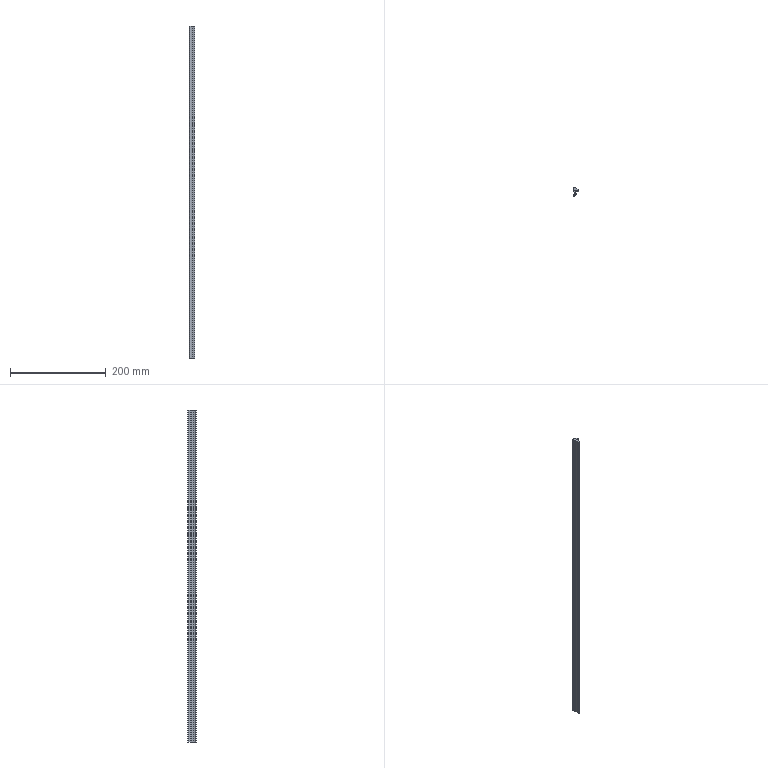Part | SolidWorks | features BaseBody 1, MoveFace 1 | 1 solid | 20 faces | box 10.8 x 17.5 x 692 mm | volume 54530 mm3 | cylinder 11 | plane 9 | commonest cylinder face diameters 1.6 x2 14 x2 0.4 x1 0.6 x1 0.8 x1 2.6 x1
STEP:
#1=CARTESIAN_POINT('',(-3.236,-11.055,592.));
#2=VERTEX_POINT('',#1);
#3=CARTESIAN_POINT('',(-4.3,-10.3,592.));
#4=VERTEX_POINT('',#3);
#5=CARTESIAN_POINT('',(-3.5,-10.3,592.));
#6=DIRECTION('',(0.,0.,-1.));
#7=DIRECTION('',(1.,0.,0.));
#8=AXIS2_PLACEMENT_3D('',#5,#6,#7);
#9=CIRCLE('',#8,0.8);
#10=EDGE_CURVE('',#2,#4,#9,.T.);
#11=ORIENTED_EDGE('',*,*,#10,.T.);
#12=CARTESIAN_POINT('',(-4.3,-10.3,-100.));
#13=VERTEX_POINT('',#12);
#14=CARTESIAN_POINT('',(-4.3,-10.3,-100.));
#15=DIRECTION('',(0.,0.,-1.));
#16=VECTOR('',#15,1000.);
#17=LINE('',#14,#16);
#18=EDGE_CURVE('',#4,#13,#17,.T.);
#19=ORIENTED_EDGE('',*,*,#18,.T.);
#20=CARTESIAN_POINT('',(-3.236,-11.055,-100.));
#21=VERTEX_POINT('',#20);
#22=CARTESIAN_POINT('',(-3.5,-10.3,-100.));
#23=DIRECTION('',(0.,0.,1.));
#24=DIRECTION('',(-1.,0.,0.));
#25=AXIS2_PLACEMENT_3D('',#22,#23,#24);
#26=CIRCLE('',#25,0.8);
#27=EDGE_CURVE('',#13,#21,#26,.T.);
#28=ORIENTED_EDGE('',*,*,#27,.T.);
#29=CARTESIAN_POINT('',(-3.236,-11.055,-100.));
#30=DIRECTION('',(0.,0.,-1.));
#31=VECTOR('',#30,1000.);
#32=LINE('',#29,#31);
#33=EDGE_CURVE('',#2,#21,#32,.T.);
#34=ORIENTED_EDGE('',*,*,#33,.F.);
#35=EDGE_LOOP('',(#11,#19,#28,#34));
#36=FACE_OUTER_BOUND('',#35,.T.);
#37=CARTESIAN_POINT('',(-3.5,-10.3,-100.));
#38=DIRECTION('',(0.,0.,-1.));
#39=DIRECTION('',(-1.,0.,0.));
#40=AXIS2_PLACEMENT_3D('',#37,#38,#39);
#41=CYLINDRICAL_SURFACE('',#40,0.8);
#42=ADVANCED_FACE('',(#36),#41,.T.);
#43=CARTESIAN_POINT('',(1.184,-6.397,-100.));
#44=VERTEX_POINT('',#43);
#45=CARTESIAN_POINT('',(-5.702,-4.29,-100.));
#46=DIRECTION('',(0.,0.,1.));
#47=DIRECTION('',(-1.,0.,0.));
#48=AXIS2_PLACEMENT_3D('',#45,#46,#47);
#49=CIRCLE('',#48,7.201);
#50=EDGE_CURVE('',#21,#44,#49,.T.);
#51=ORIENTED_EDGE('',*,*,#50,.T.);
#52=CARTESIAN_POINT('',(1.184,-6.397,592.));
#53=VERTEX_POINT('',#52);
#54=CARTESIAN_POINT('',(1.184,-6.397,-100.));
#55=DIRECTION('',(0.,0.,1.));
#56=VECTOR('',#55,1000.);
#57=LINE('',#54,#56);
#58=EDGE_CURVE('',#44,#53,#57,.T.);
#59=ORIENTED_EDGE('',*,*,#58,.T.);
#60=CARTESIAN_POINT('',(-5.702,-4.29,592.));
#61=DIRECTION('',(0.,0.,-1.));
#62=DIRECTION('',(1.,0.,0.));
#63=AXIS2_PLACEMENT_3D('',#60,#61,#62);
#64=CIRCLE('',#63,7.201);
#65=EDGE_CURVE('',#53,#2,#64,.T.);
#66=ORIENTED_EDGE('',*,*,#65,.T.);
#67=ORIENTED_EDGE('',*,*,#33,.T.);
#68=EDGE_LOOP('',(#51,#59,#66,#67));
#69=FACE_OUTER_BOUND('',#68,.T.);
#70=CARTESIAN_POINT('',(-5.702,-4.29,-100.));
#71=DIRECTION('',(0.,0.,-1.));
#72=DIRECTION('',(-1.,0.,0.));
#73=AXIS2_PLACEMENT_3D('',#70,#71,#72);
#74=CYLINDRICAL_SURFACE('',#73,7.201);
#75=ADVANCED_FACE('',(#69),#74,.T.);
#76=CARTESIAN_POINT('',(0.9,-6.,-100.));
#77=VERTEX_POINT('',#76);
#78=CARTESIAN_POINT('',(0.9,-6.3,-100.));
#79=DIRECTION('',(0.,0.,1.));
#80=DIRECTION('',(-1.,0.,0.));
#81=AXIS2_PLACEMENT_3D('',#78,#79,#80);
#82=CIRCLE('',#81,0.3);
#83=EDGE_CURVE('',#44,#77,#82,.T.);
#84=ORIENTED_EDGE('',*,*,#83,.T.);
#85=CARTESIAN_POINT('',(0.9,-6.,592.));
#86=VERTEX_POINT('',#85);
#87=CARTESIAN_POINT('',(0.9,-6.,-100.));
#88=DIRECTION('',(0.,0.,1.));
#89=VECTOR('',#88,1000.);
#90=LINE('',#87,#89);
#91=EDGE_CURVE('',#77,#86,#90,.T.);
#92=ORIENTED_EDGE('',*,*,#91,.T.);
#93=CARTESIAN_POINT('',(0.9,-6.3,592.));
#94=DIRECTION('',(0.,0.,-1.));
#95=DIRECTION('',(1.,0.,0.));
#96=AXIS2_PLACEMENT_3D('',#93,#94,#95);
#97=CIRCLE('',#96,0.3);
#98=EDGE_CURVE('',#86,#53,#97,.T.);
#99=ORIENTED_EDGE('',*,*,#98,.T.);
#100=ORIENTED_EDGE('',*,*,#58,.F.);
#101=EDGE_LOOP('',(#84,#92,#99,#100));
#102=FACE_OUTER_BOUND('',#101,.T.);
#103=CARTESIAN_POINT('',(0.9,-6.3,-100.));
#104=DIRECTION('',(0.,0.,-1.));
#105=DIRECTION('',(-1.,0.,0.));
#106=AXIS2_PLACEMENT_3D('',#103,#104,#105);
#107=CYLINDRICAL_SURFACE('',#106,0.3);
#108=ADVANCED_FACE('',(#102),#107,.T.);
#109=CARTESIAN_POINT('',(-2.5,-0.5,-100.));
#110=VERTEX_POINT('',#109);
#111=CARTESIAN_POINT('',(-2.5,-6.153,-100.));
#112=VERTEX_POINT('',#111);
#113=CARTESIAN_POINT('',(-2.5,-6.397,-100.));
#114=DIRECTION('',(0.,-1.,0.));
#115=VECTOR('',#114,1000.);
#116=LINE('',#113,#115);
#117=EDGE_CURVE('',#110,#112,#116,.T.);
#118=ORIENTED_EDGE('',*,*,#117,.F.);
#119=CARTESIAN_POINT('',(-4.2,1.695,-100.));
#120=VERTEX_POINT('',#119);
#121=CARTESIAN_POINT('',(-1.701,1.875,-100.));
#122=DIRECTION('',(0.,0.,1.));
#123=DIRECTION('',(-1.,0.,0.));
#124=AXIS2_PLACEMENT_3D('',#121,#122,#123);
#125=CIRCLE('',#124,2.506);
#126=EDGE_CURVE('',#120,#110,#125,.T.);
#127=ORIENTED_EDGE('',*,*,#126,.F.);
#128=CARTESIAN_POINT('',(-4.2,5.1,-100.));
#129=VERTEX_POINT('',#128);
#130=CARTESIAN_POINT('',(-4.2,-6.397,-100.));
#131=DIRECTION('',(0.,-1.,0.));
#132=VECTOR('',#131,1000.);
#133=LINE('',#130,#132);
#134=EDGE_CURVE('',#129,#120,#133,.T.);
#135=ORIENTED_EDGE('',*,*,#134,.F.);
#136=CARTESIAN_POINT('',(-2.892,6.4,-100.));
#137=VERTEX_POINT('',#136);
#138=CARTESIAN_POINT('',(-2.9,5.1,-100.));
#139=DIRECTION('',(0.,0.,1.));
#140=DIRECTION('',(-1.,0.,0.));
#141=AXIS2_PLACEMENT_3D('',#138,#139,#140);
#142=CIRCLE('',#141,1.3);
#143=EDGE_CURVE('',#137,#129,#142,.T.);
#144=ORIENTED_EDGE('',*,*,#143,.F.);
#145=CARTESIAN_POINT('',(0.5,5.5,-100.));
#146=VERTEX_POINT('',#145);
#147=CARTESIAN_POINT('',(-2.934,-0.5999,-100.));
#148=DIRECTION('',(0.,0.,1.));
#149=DIRECTION('',(-1.,0.,0.));
#150=AXIS2_PLACEMENT_3D('',#147,#148,#149);
#151=CIRCLE('',#150,7.);
#152=EDGE_CURVE('',#146,#137,#151,.T.);
#153=ORIENTED_EDGE('',*,*,#152,.F.);
#154=CARTESIAN_POINT('',(5.5,1.7,-100.));
#155=VERTEX_POINT('',#154);
#156=CARTESIAN_POINT('',(5.5,1.7,-100.));
#157=DIRECTION('',(-0.7962,0.6051,0.));
#158=VECTOR('',#157,1000.);
#159=LINE('',#156,#158);
#160=EDGE_CURVE('',#155,#146,#159,.T.);
#161=ORIENTED_EDGE('',*,*,#160,.F.);
#162=CARTESIAN_POINT('',(6.458,-0.2215,-100.));
#163=VERTEX_POINT('',#162);
#164=CARTESIAN_POINT('',(6.458,-0.2215,-100.));
#165=DIRECTION('',(-0.4462,0.8949,0.));
#166=VECTOR('',#165,1000.);
#167=LINE('',#164,#166);
#168=EDGE_CURVE('',#163,#155,#167,.T.);
#169=ORIENTED_EDGE('',*,*,#168,.F.);
#170=CARTESIAN_POINT('',(5.895,-0.7433,-100.));
#171=VERTEX_POINT('',#170);
#172=CARTESIAN_POINT('',(6.1,-0.4,-100.));
#173=DIRECTION('',(0.,0.,1.));
#174=DIRECTION('',(-1.,0.,0.));
#175=AXIS2_PLACEMENT_3D('',#172,#173,#174);
#176=CIRCLE('',#175,0.4);
#177=EDGE_CURVE('',#171,#163,#176,.T.);
#178=ORIENTED_EDGE('',*,*,#177,.F.);
#179=CARTESIAN_POINT('',(3.,0.,-100.));
#180=VERTEX_POINT('',#179);
#181=CARTESIAN_POINT('',(2.746,-6.995,-100.));
#182=DIRECTION('',(0.,0.,-1.));
#183=DIRECTION('',(-1.,0.,0.));
#184=AXIS2_PLACEMENT_3D('',#181,#182,#183);
#185=CIRCLE('',#184,7.);
#186=EDGE_CURVE('',#180,#171,#185,.T.);
#187=ORIENTED_EDGE('',*,*,#186,.F.);
#188=CARTESIAN_POINT('',(0.,0.,-100.));
#189=VERTEX_POINT('',#188);
#190=CARTESIAN_POINT('',(-6.814,0.,-100.));
#191=DIRECTION('',(1.,0.,0.));
#192=VECTOR('',#191,1000.);
#193=LINE('',#190,#192);
#194=EDGE_CURVE('',#189,#180,#193,.T.);
#195=ORIENTED_EDGE('',*,*,#194,.F.);
#196=CARTESIAN_POINT('',(0.,-5.8,-100.));
#197=VERTEX_POINT('',#196);
#198=CARTESIAN_POINT('',(0.,-6.397,-100.));
#199=DIRECTION('',(0.,1.,0.));
#200=VECTOR('',#199,1000.);
#201=LINE('',#198,#200);
#202=EDGE_CURVE('',#197,#189,#201,.T.);
#203=ORIENTED_EDGE('',*,*,#202,.F.);
#204=CARTESIAN_POINT('',(0.2,-6.,-100.));
#205=VERTEX_POINT('',#204);
#206=CARTESIAN_POINT('',(0.2,-5.8,-100.));
#207=DIRECTION('',(0.,0.,1.));
#208=DIRECTION('',(-1.,0.,0.));
#209=AXIS2_PLACEMENT_3D('',#206,#207,#208);
#210=CIRCLE('',#209,0.2);
#211=EDGE_CURVE('',#197,#205,#210,.T.);
#212=ORIENTED_EDGE('',*,*,#211,.T.);
#213=CARTESIAN_POINT('',(-6.814,-6.,-100.));
#214=DIRECTION('',(-1.,0.,0.));
#215=VECTOR('',#214,1000.);
#216=LINE('',#213,#215);
#217=EDGE_CURVE('',#77,#205,#216,.T.);
#218=ORIENTED_EDGE('',*,*,#217,.F.);
#219=ORIENTED_EDGE('',*,*,#83,.F.);
#220=ORIENTED_EDGE('',*,*,#50,.F.);
#221=ORIENTED_EDGE('',*,*,#27,.F.);
#222=CARTESIAN_POINT('',(-3.998,-9.674,-100.));
#223=VERTEX_POINT('',#222);
#224=CARTESIAN_POINT('',(-3.5,-10.3,-100.));
#225=DIRECTION('',(0.,0.,1.));
#226=DIRECTION('',(-1.,0.,0.));
#227=AXIS2_PLACEMENT_3D('',#224,#225,#226);
#228=CIRCLE('',#227,0.8);
#229=EDGE_CURVE('',#223,#13,#228,.T.);
#230=ORIENTED_EDGE('',*,*,#229,.F.);
#231=CARTESIAN_POINT('',(-6.814,-6.397,-100.));
#232=DIRECTION('',(0.,0.,-1.));
#233=DIRECTION('',(-1.,0.,0.));
#234=AXIS2_PLACEMENT_3D('',#231,#232,#233);
#235=CIRCLE('',#234,4.321);
#236=EDGE_CURVE('',#112,#223,#235,.T.);
#237=ORIENTED_EDGE('',*,*,#236,.F.);
#238=EDGE_LOOP('',(#118,#127,#135,#144,#153,#161,#169,#178,#187,#195,#203,#212,#218,#219,#220,#221,#230,#237));
#239=FACE_OUTER_BOUND('',#238,.T.);
#240=CARTESIAN_POINT('',(-6.814,-6.397,-100.));
#241=DIRECTION('',(0.,0.,1.));
#242=DIRECTION('',(1.,0.,0.));
#243=AXIS2_PLACEMENT_3D('',#240,#241,#242);
#244=PLANE('',#243);
#245=ADVANCED_FACE('',(#239),#244,.F.);
#246=ORIENTED_EDGE('',*,*,#18,.F.);
#247=CARTESIAN_POINT('',(-3.998,-9.674,592.));
#248=VERTEX_POINT('',#247);
#249=CARTESIAN_POINT('',(-3.5,-10.3,592.));
#250=DIRECTION('',(0.,0.,-1.));
#251=DIRECTION('',(1.,0.,0.));
#252=AXIS2_PLACEMENT_3D('',#249,#250,#251);
#253=CIRCLE('',#252,0.8);
#254=EDGE_CURVE('',#4,#248,#253,.T.);
#255=ORIENTED_EDGE('',*,*,#254,.T.);
#256=CARTESIAN_POINT('',(-3.998,-9.674,-100.));
#257=DIRECTION('',(0.,0.,-1.));
#258=VECTOR('',#257,1000.);
#259=LINE('',#256,#258);
#260=EDGE_CURVE('',#248,#223,#259,.T.);
#261=ORIENTED_EDGE('',*,*,#260,.T.);
#262=ORIENTED_EDGE('',*,*,#229,.T.);
#263=EDGE_LOOP('',(#246,#255,#261,#262));
#264=FACE_OUTER_BOUND('',#263,.T.);
#265=CARTESIAN_POINT('',(-3.5,-10.3,-100.));
#266=DIRECTION('',(0.,0.,-1.));
#267=DIRECTION('',(-1.,0.,0.));
#268=AXIS2_PLACEMENT_3D('',#265,#266,#267);
#269=CYLINDRICAL_SURFACE('',#268,0.8);
#270=ADVANCED_FACE('',(#264),#269,.T.);
#271=CARTESIAN_POINT('',(-4.2,1.695,592.));
#272=VERTEX_POINT('',#271);
#273=CARTESIAN_POINT('',(-2.5,-0.5,592.));
#274=VERTEX_POINT('',#273);
#275=CARTESIAN_POINT('',(-1.701,1.875,592.));
#276=DIRECTION('',(0.,0.,1.));
#277=DIRECTION('',(1.,0.,0.));
#278=AXIS2_PLACEMENT_3D('',#275,#276,#277);
#279=CIRCLE('',#278,2.506);
#280=EDGE_CURVE('',#272,#274,#279,.T.);
#281=ORIENTED_EDGE('',*,*,#280,.T.);
#282=CARTESIAN_POINT('',(-2.5,-6.153,592.));
#283=VERTEX_POINT('',#282);
#284=CARTESIAN_POINT('',(-2.5,-6.397,592.));
#285=DIRECTION('',(0.,-1.,0.));
#286=VECTOR('',#285,1000.);
#287=LINE('',#284,#286);
#288=EDGE_CURVE('',#274,#283,#287,.T.);
#289=ORIENTED_EDGE('',*,*,#288,.T.);
#290=CARTESIAN_POINT('',(-6.814,-6.397,592.));
#291=DIRECTION('',(0.,0.,-1.));
#292=DIRECTION('',(1.,0.,0.));
#293=AXIS2_PLACEMENT_3D('',#290,#291,#292);
#294=CIRCLE('',#293,4.321);
#295=EDGE_CURVE('',#283,#248,#294,.T.);
#296=ORIENTED_EDGE('',*,*,#295,.T.);
#297=ORIENTED_EDGE('',*,*,#254,.F.);
#298=ORIENTED_EDGE('',*,*,#10,.F.);
#299=ORIENTED_EDGE('',*,*,#65,.F.);
#300=ORIENTED_EDGE('',*,*,#98,.F.);
#301=CARTESIAN_POINT('',(0.2,-6.,592.));
#302=VERTEX_POINT('',#301);
#303=CARTESIAN_POINT('',(-6.814,-6.,592.));
#304=DIRECTION('',(-1.,0.,0.));
#305=VECTOR('',#304,1000.);
#306=LINE('',#303,#305);
#307=EDGE_CURVE('',#86,#302,#306,.T.);
#308=ORIENTED_EDGE('',*,*,#307,.T.);
#309=CARTESIAN_POINT('',(0.,-5.8,592.));
#310=VERTEX_POINT('',#309);
#311=CARTESIAN_POINT('',(0.2,-5.8,592.));
#312=DIRECTION('',(0.,0.,-1.));
#313=DIRECTION('',(1.,0.,0.));
#314=AXIS2_PLACEMENT_3D('',#311,#312,#313);
#315=CIRCLE('',#314,0.2);
#316=EDGE_CURVE('',#302,#310,#315,.T.);
#317=ORIENTED_EDGE('',*,*,#316,.T.);
#318=CARTESIAN_POINT('',(0.,0.,592.));
#319=VERTEX_POINT('',#318);
#320=CARTESIAN_POINT('',(0.,-6.397,592.));
#321=DIRECTION('',(0.,1.,0.));
#322=VECTOR('',#321,1000.);
#323=LINE('',#320,#322);
#324=EDGE_CURVE('',#310,#319,#323,.T.);
#325=ORIENTED_EDGE('',*,*,#324,.T.);
#326=CARTESIAN_POINT('',(3.,0.,592.));
#327=VERTEX_POINT('',#326);
#328=CARTESIAN_POINT('',(-6.814,0.,592.));
#329=DIRECTION('',(1.,0.,0.));
#330=VECTOR('',#329,1000.);
#331=LINE('',#328,#330);
#332=EDGE_CURVE('',#319,#327,#331,.T.);
#333=ORIENTED_EDGE('',*,*,#332,.T.);
#334=CARTESIAN_POINT('',(5.895,-0.7433,592.));
#335=VERTEX_POINT('',#334);
#336=CARTESIAN_POINT('',(2.746,-6.995,592.));
#337=DIRECTION('',(0.,0.,-1.));
#338=DIRECTION('',(1.,0.,0.));
#339=AXIS2_PLACEMENT_3D('',#336,#337,#338);
#340=CIRCLE('',#339,7.);
#341=EDGE_CURVE('',#327,#335,#340,.T.);
#342=ORIENTED_EDGE('',*,*,#341,.T.);
#343=CARTESIAN_POINT('',(6.458,-0.2215,592.));
#344=VERTEX_POINT('',#343);
#345=CARTESIAN_POINT('',(6.1,-0.4,592.));
#346=DIRECTION('',(0.,0.,-1.));
#347=DIRECTION('',(1.,0.,0.));
#348=AXIS2_PLACEMENT_3D('',#345,#346,#347);
#349=CIRCLE('',#348,0.4);
#350=EDGE_CURVE('',#344,#335,#349,.T.);
#351=ORIENTED_EDGE('',*,*,#350,.F.);
#352=CARTESIAN_POINT('',(5.5,1.7,592.));
#353=VERTEX_POINT('',#352);
#354=CARTESIAN_POINT('',(6.282,0.1323,592.));
#355=DIRECTION('',(-0.4462,0.8949,0.));
#356=VECTOR('',#355,1000.);
#357=LINE('',#354,#356);
#358=EDGE_CURVE('',#344,#353,#357,.T.);
#359=ORIENTED_EDGE('',*,*,#358,.T.);
#360=CARTESIAN_POINT('',(0.5,5.5,592.));
#361=VERTEX_POINT('',#360);
#362=CARTESIAN_POINT('',(1.595,4.668,592.));
#363=DIRECTION('',(-0.7962,0.6051,0.));
#364=VECTOR('',#363,1000.);
#365=LINE('',#362,#364);
#366=EDGE_CURVE('',#353,#361,#365,.T.);
#367=ORIENTED_EDGE('',*,*,#366,.T.);
#368=CARTESIAN_POINT('',(-2.892,6.4,592.));
#369=VERTEX_POINT('',#368);
#370=CARTESIAN_POINT('',(-2.934,-0.5999,592.));
#371=DIRECTION('',(0.,0.,1.));
#372=DIRECTION('',(1.,0.,0.));
#373=AXIS2_PLACEMENT_3D('',#370,#371,#372);
#374=CIRCLE('',#373,7.);
#375=EDGE_CURVE('',#361,#369,#374,.T.);
#376=ORIENTED_EDGE('',*,*,#375,.T.);
#377=CARTESIAN_POINT('',(-4.2,5.1,592.));
#378=VERTEX_POINT('',#377);
#379=CARTESIAN_POINT('',(-2.9,5.1,592.));
#380=DIRECTION('',(0.,0.,1.));
#381=DIRECTION('',(1.,0.,0.));
#382=AXIS2_PLACEMENT_3D('',#379,#380,#381);
#383=CIRCLE('',#382,1.3);
#384=EDGE_CURVE('',#369,#378,#383,.T.);
#385=ORIENTED_EDGE('',*,*,#384,.T.);
#386=CARTESIAN_POINT('',(-4.2,-6.397,592.));
#387=DIRECTION('',(0.,-1.,0.));
#388=VECTOR('',#387,1000.);
#389=LINE('',#386,#388);
#390=EDGE_CURVE('',#378,#272,#389,.T.);
#391=ORIENTED_EDGE('',*,*,#390,.T.);
#392=EDGE_LOOP('',(#281,#289,#296,#297,#298,#299,#300,#308,#317,#325,#333,#342,#351,#359,#367,#376,#385,#391));
#393=FACE_OUTER_BOUND('',#392,.T.);
#394=CARTESIAN_POINT('',(-6.814,-6.397,592.));
#395=DIRECTION('',(0.,0.,1.));
#396=DIRECTION('',(1.,0.,0.));
#397=AXIS2_PLACEMENT_3D('',#394,#395,#396);
#398=PLANE('',#397);
#399=ADVANCED_FACE('',(#393),#398,.T.);
#400=ORIENTED_EDGE('',*,*,#217,.T.);
#401=CARTESIAN_POINT('',(0.2,-6.,-100.));
#402=DIRECTION('',(0.,0.,1.));
#403=VECTOR('',#402,1000.);
#404=LINE('',#401,#403);
#405=EDGE_CURVE('',#205,#302,#404,.T.);
#406=ORIENTED_EDGE('',*,*,#405,.T.);
#407=ORIENTED_EDGE('',*,*,#307,.F.);
#408=ORIENTED_EDGE('',*,*,#91,.F.);
#409=EDGE_LOOP('',(#400,#406,#407,#408));
#410=FACE_OUTER_BOUND('',#409,.T.);
#411=CARTESIAN_POINT('',(0.9,-6.,-100.));
#412=DIRECTION('',(0.,1.,0.));
#413=DIRECTION('',(0.,0.,1.));
#414=AXIS2_PLACEMENT_3D('',#411,#412,#413);
#415=PLANE('',#414);
#416=ADVANCED_FACE('',(#410),#415,.T.);
#417=CARTESIAN_POINT('',(-2.5,-6.153,-100.));
#418=DIRECTION('',(0.,0.,1.));
#419=VECTOR('',#418,1000.);
#420=LINE('',#417,#419);
#421=EDGE_CURVE('',#112,#283,#420,.T.);
#422=ORIENTED_EDGE('',*,*,#421,.F.);
#423=ORIENTED_EDGE('',*,*,#236,.T.);
#424=ORIENTED_EDGE('',*,*,#260,.F.);
#425=ORIENTED_EDGE('',*,*,#295,.F.);
#426=EDGE_LOOP('',(#422,#423,#424,#425));
#427=FACE_OUTER_BOUND('',#426,.T.);
#428=CARTESIAN_POINT('',(-6.814,-6.397,-100.));
#429=DIRECTION('',(0.,0.,-1.));
#430=DIRECTION('',(-1.,0.,0.));
#431=AXIS2_PLACEMENT_3D('',#428,#429,#430);
#432=CYLINDRICAL_SURFACE('',#431,4.321);
#433=ADVANCED_FACE('',(#427),#432,.F.);
#434=ORIENTED_EDGE('',*,*,#117,.T.);
#435=ORIENTED_EDGE('',*,*,#421,.T.);
#436=ORIENTED_EDGE('',*,*,#288,.F.);
#437=CARTESIAN_POINT('',(-2.5,-0.5,-100.));
#438=DIRECTION('',(0.,0.,-1.));
#439=VECTOR('',#438,1000.);
#440=LINE('',#437,#439);
#441=EDGE_CURVE('',#274,#110,#440,.T.);
#442=ORIENTED_EDGE('',*,*,#441,.T.);
#443=EDGE_LOOP('',(#434,#435,#436,#442));
#444=FACE_OUTER_BOUND('',#443,.T.);
#445=CARTESIAN_POINT('',(-2.5,-0.5,-100.));
#446=DIRECTION('',(-1.,0.,0.));
#447=DIRECTION('',(0.,0.,1.));
#448=AXIS2_PLACEMENT_3D('',#445,#446,#447);
#449=PLANE('',#448);
#450=ADVANCED_FACE('',(#444),#449,.T.);
#451=ORIENTED_EDGE('',*,*,#126,.T.);
#452=ORIENTED_EDGE('',*,*,#441,.F.);
#453=ORIENTED_EDGE('',*,*,#280,.F.);
#454=CARTESIAN_POINT('',(-4.2,1.695,-100.));
#455=DIRECTION('',(0.,0.,-1.));
#456=VECTOR('',#455,1000.);
#457=LINE('',#454,#456);
#458=EDGE_CURVE('',#272,#120,#457,.T.);
#459=ORIENTED_EDGE('',*,*,#458,.T.);
#460=EDGE_LOOP('',(#451,#452,#453,#459));
#461=FACE_OUTER_BOUND('',#460,.T.);
#462=CARTESIAN_POINT('',(-1.701,1.875,-100.));
#463=DIRECTION('',(0.,0.,-1.));
#464=DIRECTION('',(-1.,0.,0.));
#465=AXIS2_PLACEMENT_3D('',#462,#463,#464);
#466=CYLINDRICAL_SURFACE('',#465,2.506);
#467=ADVANCED_FACE('',(#461),#466,.T.);
#468=ORIENTED_EDGE('',*,*,#134,.T.);
#469=ORIENTED_EDGE('',*,*,#458,.F.);
#470=ORIENTED_EDGE('',*,*,#390,.F.);
#471=CARTESIAN_POINT('',(-4.2,5.1,-100.));
#472=DIRECTION('',(0.,0.,-1.));
#473=VECTOR('',#472,1000.);
#474=LINE('',#471,#473);
#475=EDGE_CURVE('',#378,#129,#474,.T.);
#476=ORIENTED_EDGE('',*,*,#475,.T.);
#477=EDGE_LOOP('',(#468,#469,#470,#476));
#478=FACE_OUTER_BOUND('',#477,.T.);
#479=CARTESIAN_POINT('',(-4.2,5.1,-100.));
#480=DIRECTION('',(-1.,0.,0.));
#481=DIRECTION('',(0.,0.,1.));
#482=AXIS2_PLACEMENT_3D('',#479,#480,#481);
#483=PLANE('',#482);
#484=ADVANCED_FACE('',(#478),#483,.T.);
#485=ORIENTED_EDGE('',*,*,#143,.T.);
#486=ORIENTED_EDGE('',*,*,#475,.F.);
#487=ORIENTED_EDGE('',*,*,#384,.F.);
#488=CARTESIAN_POINT('',(-2.892,6.4,-100.));
#489=DIRECTION('',(0.,0.,-1.));
#490=VECTOR('',#489,1000.);
#491=LINE('',#488,#490);
#492=EDGE_CURVE('',#369,#137,#491,.T.);
#493=ORIENTED_EDGE('',*,*,#492,.T.);
#494=EDGE_LOOP('',(#485,#486,#487,#493));
#495=FACE_OUTER_BOUND('',#494,.T.);
#496=CARTESIAN_POINT('',(-2.9,5.1,-100.));
#497=DIRECTION('',(0.,0.,-1.));
#498=DIRECTION('',(-1.,0.,0.));
#499=AXIS2_PLACEMENT_3D('',#496,#497,#498);
#500=CYLINDRICAL_SURFACE('',#499,1.3);
#501=ADVANCED_FACE('',(#495),#500,.T.);
#502=ORIENTED_EDGE('',*,*,#152,.T.);
#503=ORIENTED_EDGE('',*,*,#492,.F.);
#504=ORIENTED_EDGE('',*,*,#375,.F.);
#505=CARTESIAN_POINT('',(0.5,5.5,-100.));
#506=DIRECTION('',(0.,0.,-1.));
#507=VECTOR('',#506,1000.);
#508=LINE('',#505,#507);
#509=EDGE_CURVE('',#361,#146,#508,.T.);
#510=ORIENTED_EDGE('',*,*,#509,.T.);
#511=EDGE_LOOP('',(#502,#503,#504,#510));
#512=FACE_OUTER_BOUND('',#511,.T.);
#513=CARTESIAN_POINT('',(-2.934,-0.5999,-100.));
#514=DIRECTION('',(0.,0.,-1.));
#515=DIRECTION('',(-1.,0.,0.));
#516=AXIS2_PLACEMENT_3D('',#513,#514,#515);
#517=CYLINDRICAL_SURFACE('',#516,7.);
#518=ADVANCED_FACE('',(#512),#517,.T.);
#519=ORIENTED_EDGE('',*,*,#160,.T.);
#520=ORIENTED_EDGE('',*,*,#509,.F.);
#521=ORIENTED_EDGE('',*,*,#366,.F.);
#522=CARTESIAN_POINT('',(5.5,1.7,-100.));
#523=DIRECTION('',(0.,0.,-1.));
#524=VECTOR('',#523,1000.);
#525=LINE('',#522,#524);
#526=EDGE_CURVE('',#353,#155,#525,.T.);
#527=ORIENTED_EDGE('',*,*,#526,.T.);
#528=EDGE_LOOP('',(#519,#520,#521,#527));
#529=FACE_OUTER_BOUND('',#528,.T.);
#530=CARTESIAN_POINT('',(5.5,1.7,-100.));
#531=DIRECTION('',(0.6051,0.7962,0.));
#532=DIRECTION('',(-0.7962,0.6051,0.));
#533=AXIS2_PLACEMENT_3D('',#530,#531,#532);
#534=PLANE('',#533);
#535=ADVANCED_FACE('',(#529),#534,.T.);
#536=ORIENTED_EDGE('',*,*,#168,.T.);
#537=ORIENTED_EDGE('',*,*,#526,.F.);
#538=ORIENTED_EDGE('',*,*,#358,.F.);
#539=CARTESIAN_POINT('',(6.458,-0.2215,-100.));
#540=DIRECTION('',(0.,0.,-1.));
#541=VECTOR('',#540,1000.);
#542=LINE('',#539,#541);
#543=EDGE_CURVE('',#344,#163,#542,.T.);
#544=ORIENTED_EDGE('',*,*,#543,.T.);
#545=EDGE_LOOP('',(#536,#537,#538,#544));
#546=FACE_OUTER_BOUND('',#545,.T.);
#547=CARTESIAN_POINT('',(6.458,-0.2215,-100.));
#548=DIRECTION('',(0.8949,0.4462,0.));
#549=DIRECTION('',(-0.4462,0.8949,0.));
#550=AXIS2_PLACEMENT_3D('',#547,#548,#549);
#551=PLANE('',#550);
#552=ADVANCED_FACE('',(#546),#551,.T.);
#553=CARTESIAN_POINT('',(3.,0.,-100.));
#554=DIRECTION('',(0.,0.,1.));
#555=VECTOR('',#554,1000.);
#556=LINE('',#553,#555);
#557=EDGE_CURVE('',#180,#327,#556,.T.);
#558=ORIENTED_EDGE('',*,*,#557,.F.);
#559=ORIENTED_EDGE('',*,*,#186,.T.);
#560=CARTESIAN_POINT('',(5.895,-0.7433,-100.));
#561=DIRECTION('',(0.,0.,-1.));
#562=VECTOR('',#561,1000.);
#563=LINE('',#560,#562);
#564=EDGE_CURVE('',#335,#171,#563,.T.);
#565=ORIENTED_EDGE('',*,*,#564,.F.);
#566=ORIENTED_EDGE('',*,*,#341,.F.);
#567=EDGE_LOOP('',(#558,#559,#565,#566));
#568=FACE_OUTER_BOUND('',#567,.T.);
#569=CARTESIAN_POINT('',(2.746,-6.995,-100.));
#570=DIRECTION('',(0.,0.,-1.));
#571=DIRECTION('',(-1.,0.,0.));
#572=AXIS2_PLACEMENT_3D('',#569,#570,#571);
#573=CYLINDRICAL_SURFACE('',#572,7.);
#574=ADVANCED_FACE('',(#568),#573,.F.);
#575=ORIENTED_EDGE('',*,*,#194,.T.);
#576=ORIENTED_EDGE('',*,*,#557,.T.);
#577=ORIENTED_EDGE('',*,*,#332,.F.);
#578=CARTESIAN_POINT('',(0.,0.,-100.));
#579=DIRECTION('',(0.,0.,-1.));
#580=VECTOR('',#579,1000.);
#581=LINE('',#578,#580);
#582=EDGE_CURVE('',#319,#189,#581,.T.);
#583=ORIENTED_EDGE('',*,*,#582,.T.);
#584=EDGE_LOOP('',(#575,#576,#577,#583));
#585=FACE_OUTER_BOUND('',#584,.T.);
#586=CARTESIAN_POINT('',(0.,0.,-100.));
#587=DIRECTION('',(0.,-1.,0.));
#588=DIRECTION('',(0.,0.,-1.));
#589=AXIS2_PLACEMENT_3D('',#586,#587,#588);
#590=PLANE('',#589);
#591=ADVANCED_FACE('',(#585),#590,.T.);
#592=ORIENTED_EDGE('',*,*,#202,.T.);
#593=ORIENTED_EDGE('',*,*,#582,.F.);
#594=ORIENTED_EDGE('',*,*,#324,.F.);
#595=CARTESIAN_POINT('',(0.,-5.8,-100.));
#596=DIRECTION('',(0.,0.,-1.));
#597=VECTOR('',#596,1000.);
#598=LINE('',#595,#597);
#599=EDGE_CURVE('',#310,#197,#598,.T.);
#600=ORIENTED_EDGE('',*,*,#599,.T.);
#601=EDGE_LOOP('',(#592,#593,#594,#600));
#602=FACE_OUTER_BOUND('',#601,.T.);
#603=CARTESIAN_POINT('',(0.,-5.8,-100.));
#604=DIRECTION('',(1.,0.,0.));
#605=DIRECTION('',(0.,0.,-1.));
#606=AXIS2_PLACEMENT_3D('',#603,#604,#605);
#607=PLANE('',#606);
#608=ADVANCED_FACE('',(#602),#607,.T.);
#609=ORIENTED_EDGE('',*,*,#405,.F.);
#610=ORIENTED_EDGE('',*,*,#211,.F.);
#611=ORIENTED_EDGE('',*,*,#599,.F.);
#612=ORIENTED_EDGE('',*,*,#316,.F.);
#613=EDGE_LOOP('',(#609,#610,#611,#612));
#614=FACE_OUTER_BOUND('',#613,.T.);
#615=CARTESIAN_POINT('',(0.2,-5.8,-100.));
#616=DIRECTION('',(0.,0.,-1.));
#617=DIRECTION('',(-1.,0.,0.));
#618=AXIS2_PLACEMENT_3D('',#615,#616,#617);
#619=CYLINDRICAL_SURFACE('',#618,0.2);
#620=ADVANCED_FACE('',(#614),#619,.F.);
#621=ORIENTED_EDGE('',*,*,#177,.T.);
#622=ORIENTED_EDGE('',*,*,#543,.F.);
#623=ORIENTED_EDGE('',*,*,#350,.T.);
#624=ORIENTED_EDGE('',*,*,#564,.T.);
#625=EDGE_LOOP('',(#621,#622,#623,#624));
#626=FACE_OUTER_BOUND('',#625,.T.);
#627=CARTESIAN_POINT('',(6.1,-0.4,-100.));
#628=DIRECTION('',(0.,0.,-1.));
#629=DIRECTION('',(-1.,0.,0.));
#630=AXIS2_PLACEMENT_3D('',#627,#628,#629);
#631=CYLINDRICAL_SURFACE('',#630,0.4);
#632=ADVANCED_FACE('',(#626),#631,.T.);
#633=CLOSED_SHELL('',(#42,#75,#108,#245,#270,#399,#416,#433,#450,#467,#484,#501,#518,#535,#552,#574,#591,#608,#620,#632));
#634=MANIFOLD_SOLID_BREP('',#633);
#635=CARTESIAN_POINT('',(0.,0.,0.));
#636=DIRECTION('',(0.,0.,1.));
#637=DIRECTION('',(1.,0.,0.));
#638=AXIS2_PLACEMENT_3D('',#635,#636,#637);
#639=(LENGTH_UNIT()NAMED_UNIT(*)SI_UNIT(.MILLI.,.METRE.));
#640=UNCERTAINTY_MEASURE_WITH_UNIT(LENGTH_MEASURE(0.00001),#639,'','');
#641=(NAMED_UNIT(*)PLANE_ANGLE_UNIT()SI_UNIT($,.RADIAN.));
#642=(NAMED_UNIT(*)SI_UNIT($,.STERADIAN.)SOLID_ANGLE_UNIT());
#643=(GEOMETRIC_REPRESENTATION_CONTEXT(3)GLOBAL_UNCERTAINTY_ASSIGNED_CONTEXT((#640))GLOBAL_UNIT_ASSIGNED_CONTEXT((#639,#641,#642))REPRESENTATION_CONTEXT('',''));
#644=ADVANCED_BREP_SHAPE_REPRESENTATION('',(#634,#638),#643);